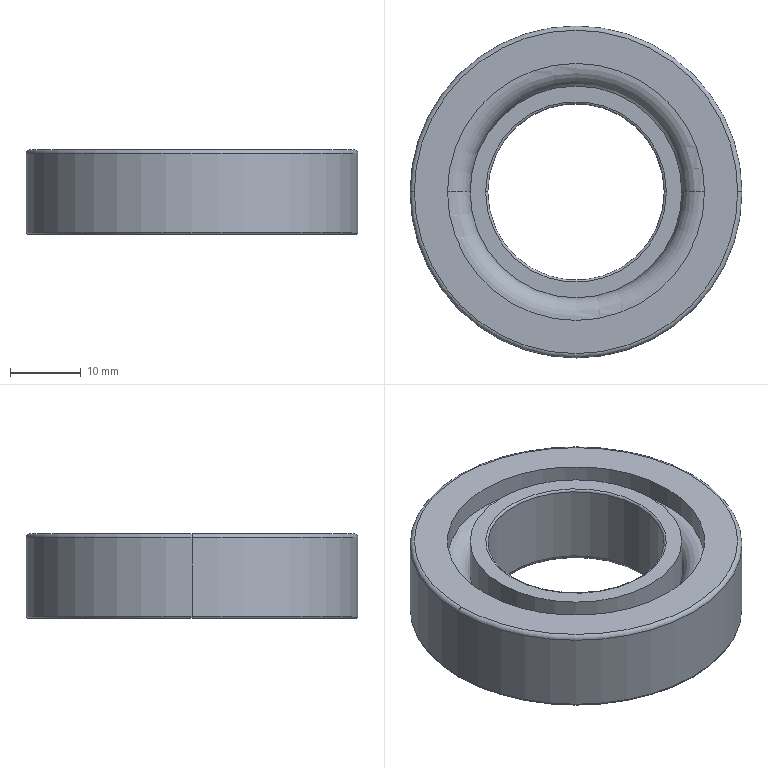Part | SolidWorks | features BaseBody 1 | 1 solid | 28 faces | box 47 x 47 x 12 mm | volume 12629 mm3 | torus 12 | cylinder 12 | plane 4 | commonest cylinder face diameters 25 x2 30 x2 36.4 x2 37.5 x2 42 x2 47 x2
STEP:
#1=CARTESIAN_POINT('',(-23.5,0.,-11.7));
#2=VERTEX_POINT('',#1);
#3=CARTESIAN_POINT('',(23.5,0.,-11.7));
#4=VERTEX_POINT('',#3);
#5=CARTESIAN_POINT('',(0.,0.,-11.7));
#6=DIRECTION('',(0.,0.,-1.));
#7=DIRECTION('',(-1.,0.,0.));
#8=AXIS2_PLACEMENT_3D('',#5,#6,#7);
#9=CIRCLE('',#8,23.5);
#10=EDGE_CURVE('',#2,#4,#9,.T.);
#11=ORIENTED_EDGE('',*,*,#10,.T.);
#12=CARTESIAN_POINT('',(23.2,0.,-12.));
#13=VERTEX_POINT('',#12);
#14=CARTESIAN_POINT('',(23.2,0.,-11.7));
#15=DIRECTION('',(0.,1.,0.));
#16=DIRECTION('',(-1.,0.,0.));
#17=AXIS2_PLACEMENT_3D('',#14,#15,#16);
#18=CIRCLE('',#17,0.3);
#19=EDGE_CURVE('',#4,#13,#18,.T.);
#20=ORIENTED_EDGE('',*,*,#19,.T.);
#21=CARTESIAN_POINT('',(-23.2,0.,-12.));
#22=VERTEX_POINT('',#21);
#23=CARTESIAN_POINT('',(0.,0.,-12.));
#24=DIRECTION('',(0.,0.,-1.));
#25=DIRECTION('',(-1.,0.,0.));
#26=AXIS2_PLACEMENT_3D('',#23,#24,#25);
#27=CIRCLE('',#26,23.2);
#28=EDGE_CURVE('',#22,#13,#27,.T.);
#29=ORIENTED_EDGE('',*,*,#28,.F.);
#30=CARTESIAN_POINT('',(-23.2,0.,-11.7));
#31=DIRECTION('',(0.,-1.,0.));
#32=DIRECTION('',(0.,0.,-1.));
#33=AXIS2_PLACEMENT_3D('',#30,#31,#32);
#34=CIRCLE('',#33,0.3);
#35=EDGE_CURVE('',#2,#22,#34,.T.);
#36=ORIENTED_EDGE('',*,*,#35,.F.);
#37=EDGE_LOOP('',(#11,#20,#29,#36));
#38=FACE_OUTER_BOUND('',#37,.T.);
#39=CARTESIAN_POINT('',(0.,0.,-11.7));
#40=DIRECTION('',(0.,0.,-1.));
#41=DIRECTION('',(-1.,0.,0.));
#42=AXIS2_PLACEMENT_3D('',#39,#40,#41);
#43=TOROIDAL_SURFACE('',#42,23.2,0.3);
#44=ADVANCED_FACE('',(#38),#43,.T.);
#45=CARTESIAN_POINT('',(21.,0.,-6.));
#46=VERTEX_POINT('',#45);
#47=CARTESIAN_POINT('',(-21.,0.,-6.));
#48=VERTEX_POINT('',#47);
#49=CARTESIAN_POINT('',(0.,0.,-6.));
#50=DIRECTION('',(0.,0.,-1.));
#51=DIRECTION('',(-1.,0.,0.));
#52=AXIS2_PLACEMENT_3D('',#49,#50,#51);
#53=CIRCLE('',#52,21.);
#54=EDGE_CURVE('',#46,#48,#53,.T.);
#55=ORIENTED_EDGE('',*,*,#54,.F.);
#56=CARTESIAN_POINT('',(21.,0.,-12.));
#57=VERTEX_POINT('',#56);
#58=CARTESIAN_POINT('',(21.,0.,-12.));
#59=DIRECTION('',(0.,0.,-1.));
#60=VECTOR('',#59,1000.);
#61=LINE('',#58,#60);
#62=EDGE_CURVE('',#46,#57,#61,.T.);
#63=ORIENTED_EDGE('',*,*,#62,.T.);
#64=CARTESIAN_POINT('',(-21.,0.,-12.));
#65=VERTEX_POINT('',#64);
#66=CARTESIAN_POINT('',(0.,0.,-12.));
#67=DIRECTION('',(0.,0.,-1.));
#68=DIRECTION('',(-1.,0.,0.));
#69=AXIS2_PLACEMENT_3D('',#66,#67,#68);
#70=CIRCLE('',#69,21.);
#71=EDGE_CURVE('',#57,#65,#70,.T.);
#72=ORIENTED_EDGE('',*,*,#71,.T.);
#73=CARTESIAN_POINT('',(-21.,0.,-12.));
#74=DIRECTION('',(0.,0.,-1.));
#75=VECTOR('',#74,1000.);
#76=LINE('',#73,#75);
#77=EDGE_CURVE('',#48,#65,#76,.T.);
#78=ORIENTED_EDGE('',*,*,#77,.F.);
#79=EDGE_LOOP('',(#55,#63,#72,#78));
#80=FACE_OUTER_BOUND('',#79,.T.);
#81=CARTESIAN_POINT('',(0.,0.,-12.));
#82=DIRECTION('',(0.,0.,-1.));
#83=DIRECTION('',(-1.,0.,0.));
#84=AXIS2_PLACEMENT_3D('',#81,#82,#83);
#85=CYLINDRICAL_SURFACE('',#84,21.);
#86=ADVANCED_FACE('',(#80),#85,.F.);
#87=CARTESIAN_POINT('',(-23.5,0.,-0.6));
#88=VERTEX_POINT('',#87);
#89=CARTESIAN_POINT('',(23.5,0.,-0.6));
#90=VERTEX_POINT('',#89);
#91=CARTESIAN_POINT('',(0.,0.,-0.6));
#92=DIRECTION('',(0.,0.,-1.));
#93=DIRECTION('',(-1.,0.,0.));
#94=AXIS2_PLACEMENT_3D('',#91,#92,#93);
#95=CIRCLE('',#94,23.5);
#96=EDGE_CURVE('',#88,#90,#95,.T.);
#97=ORIENTED_EDGE('',*,*,#96,.T.);
#98=CARTESIAN_POINT('',(23.5,0.,-12.));
#99=DIRECTION('',(0.,0.,-1.));
#100=VECTOR('',#99,1000.);
#101=LINE('',#98,#100);
#102=EDGE_CURVE('',#90,#4,#101,.T.);
#103=ORIENTED_EDGE('',*,*,#102,.T.);
#104=ORIENTED_EDGE('',*,*,#10,.F.);
#105=CARTESIAN_POINT('',(-23.5,0.,-12.));
#106=DIRECTION('',(0.,0.,-1.));
#107=VECTOR('',#106,1000.);
#108=LINE('',#105,#107);
#109=EDGE_CURVE('',#88,#2,#108,.T.);
#110=ORIENTED_EDGE('',*,*,#109,.F.);
#111=EDGE_LOOP('',(#97,#103,#104,#110));
#112=FACE_OUTER_BOUND('',#111,.T.);
#113=CARTESIAN_POINT('',(0.,0.,-12.));
#114=DIRECTION('',(0.,0.,-1.));
#115=DIRECTION('',(-1.,0.,0.));
#116=AXIS2_PLACEMENT_3D('',#113,#114,#115);
#117=CYLINDRICAL_SURFACE('',#116,23.5);
#118=ADVANCED_FACE('',(#112),#117,.T.);
#119=CARTESIAN_POINT('',(0.,0.,-6.));
#120=DIRECTION('',(0.,0.,-1.));
#121=DIRECTION('',(-1.,0.,0.));
#122=AXIS2_PLACEMENT_3D('',#119,#120,#121);
#123=CIRCLE('',#122,21.);
#124=EDGE_CURVE('',#48,#46,#123,.T.);
#125=ORIENTED_EDGE('',*,*,#124,.T.);
#126=CARTESIAN_POINT('',(18.75,0.,-8.905));
#127=VERTEX_POINT('',#126);
#128=CARTESIAN_POINT('',(18.,0.,-6.));
#129=DIRECTION('',(0.,1.,0.));
#130=DIRECTION('',(-1.,0.,0.));
#131=AXIS2_PLACEMENT_3D('',#128,#129,#130);
#132=CIRCLE('',#131,3.);
#133=EDGE_CURVE('',#46,#127,#132,.T.);
#134=ORIENTED_EDGE('',*,*,#133,.T.);
#135=CARTESIAN_POINT('',(-18.75,0.,-8.905));
#136=VERTEX_POINT('',#135);
#137=CARTESIAN_POINT('',(0.,0.,-8.905));
#138=DIRECTION('',(0.,0.,-1.));
#139=DIRECTION('',(-1.,0.,0.));
#140=AXIS2_PLACEMENT_3D('',#137,#138,#139);
#141=CIRCLE('',#140,18.75);
#142=EDGE_CURVE('',#136,#127,#141,.T.);
#143=ORIENTED_EDGE('',*,*,#142,.F.);
#144=CARTESIAN_POINT('',(-18.,0.,-6.));
#145=DIRECTION('',(0.,-1.,0.));
#146=DIRECTION('',(0.,0.,-1.));
#147=AXIS2_PLACEMENT_3D('',#144,#145,#146);
#148=CIRCLE('',#147,3.);
#149=EDGE_CURVE('',#48,#136,#148,.T.);
#150=ORIENTED_EDGE('',*,*,#149,.F.);
#151=EDGE_LOOP('',(#125,#134,#143,#150));
#152=FACE_OUTER_BOUND('',#151,.T.);
#153=CARTESIAN_POINT('',(0.,0.,-6.));
#154=DIRECTION('',(0.,0.,-1.));
#155=DIRECTION('',(-1.,0.,0.));
#156=AXIS2_PLACEMENT_3D('',#153,#154,#155);
#157=TOROIDAL_SURFACE('',#156,18.,3.);
#158=ADVANCED_FACE('',(#152),#157,.T.);
#159=CARTESIAN_POINT('',(-22.9,0.,0.));
#160=VERTEX_POINT('',#159);
#161=CARTESIAN_POINT('',(22.9,0.,0.));
#162=VERTEX_POINT('',#161);
#163=CARTESIAN_POINT('',(0.,0.,0.));
#164=DIRECTION('',(0.,0.,-1.));
#165=DIRECTION('',(-1.,0.,0.));
#166=AXIS2_PLACEMENT_3D('',#163,#164,#165);
#167=CIRCLE('',#166,22.9);
#168=EDGE_CURVE('',#160,#162,#167,.T.);
#169=ORIENTED_EDGE('',*,*,#168,.T.);
#170=CARTESIAN_POINT('',(22.9,0.,-0.6));
#171=DIRECTION('',(0.,1.,0.));
#172=DIRECTION('',(-1.,0.,0.));
#173=AXIS2_PLACEMENT_3D('',#170,#171,#172);
#174=CIRCLE('',#173,0.6);
#175=EDGE_CURVE('',#162,#90,#174,.T.);
#176=ORIENTED_EDGE('',*,*,#175,.T.);
#177=ORIENTED_EDGE('',*,*,#96,.F.);
#178=CARTESIAN_POINT('',(-22.9,0.,-0.6));
#179=DIRECTION('',(0.,-1.,0.));
#180=DIRECTION('',(0.,0.,-1.));
#181=AXIS2_PLACEMENT_3D('',#178,#179,#180);
#182=CIRCLE('',#181,0.6);
#183=EDGE_CURVE('',#160,#88,#182,.T.);
#184=ORIENTED_EDGE('',*,*,#183,.F.);
#185=EDGE_LOOP('',(#169,#176,#177,#184));
#186=FACE_OUTER_BOUND('',#185,.T.);
#187=CARTESIAN_POINT('',(0.,0.,-0.6));
#188=DIRECTION('',(0.,0.,-1.));
#189=DIRECTION('',(-1.,0.,0.));
#190=AXIS2_PLACEMENT_3D('',#187,#188,#189);
#191=TOROIDAL_SURFACE('',#190,22.9,0.6);
#192=ADVANCED_FACE('',(#186),#191,.T.);
#193=ORIENTED_EDGE('',*,*,#142,.T.);
#194=CARTESIAN_POINT('',(18.75,0.,-12.));
#195=VERTEX_POINT('',#194);
#196=CARTESIAN_POINT('',(18.75,0.,-12.));
#197=DIRECTION('',(0.,0.,-1.));
#198=VECTOR('',#197,1000.);
#199=LINE('',#196,#198);
#200=EDGE_CURVE('',#127,#195,#199,.T.);
#201=ORIENTED_EDGE('',*,*,#200,.T.);
#202=CARTESIAN_POINT('',(-18.75,0.,-12.));
#203=VERTEX_POINT('',#202);
#204=CARTESIAN_POINT('',(0.,0.,-12.));
#205=DIRECTION('',(0.,0.,-1.));
#206=DIRECTION('',(-1.,0.,0.));
#207=AXIS2_PLACEMENT_3D('',#204,#205,#206);
#208=CIRCLE('',#207,18.75);
#209=EDGE_CURVE('',#203,#195,#208,.T.);
#210=ORIENTED_EDGE('',*,*,#209,.F.);
#211=CARTESIAN_POINT('',(-18.75,0.,-12.));
#212=DIRECTION('',(0.,0.,-1.));
#213=VECTOR('',#212,1000.);
#214=LINE('',#211,#213);
#215=EDGE_CURVE('',#136,#203,#214,.T.);
#216=ORIENTED_EDGE('',*,*,#215,.F.);
#217=EDGE_LOOP('',(#193,#201,#210,#216));
#218=FACE_OUTER_BOUND('',#217,.T.);
#219=CARTESIAN_POINT('',(0.,0.,-12.));
#220=DIRECTION('',(0.,0.,-1.));
#221=DIRECTION('',(-1.,0.,0.));
#222=AXIS2_PLACEMENT_3D('',#219,#220,#221);
#223=CYLINDRICAL_SURFACE('',#222,18.75);
#224=ADVANCED_FACE('',(#218),#223,.T.);
#225=CARTESIAN_POINT('',(18.2,0.,0.));
#226=VERTEX_POINT('',#225);
#227=CARTESIAN_POINT('',(-18.2,0.,0.));
#228=VERTEX_POINT('',#227);
#229=CARTESIAN_POINT('',(0.,0.,0.));
#230=DIRECTION('',(0.,0.,-1.));
#231=DIRECTION('',(-1.,0.,0.));
#232=AXIS2_PLACEMENT_3D('',#229,#230,#231);
#233=CIRCLE('',#232,18.2);
#234=EDGE_CURVE('',#226,#228,#233,.T.);
#235=ORIENTED_EDGE('',*,*,#234,.F.);
#236=CARTESIAN_POINT('',(18.2,0.,-3.007));
#237=VERTEX_POINT('',#236);
#238=CARTESIAN_POINT('',(18.2,0.,-12.));
#239=DIRECTION('',(0.,0.,-1.));
#240=VECTOR('',#239,1000.);
#241=LINE('',#238,#240);
#242=EDGE_CURVE('',#226,#237,#241,.T.);
#243=ORIENTED_EDGE('',*,*,#242,.T.);
#244=CARTESIAN_POINT('',(-18.2,0.,-3.007));
#245=VERTEX_POINT('',#244);
#246=CARTESIAN_POINT('',(0.,0.,-3.007));
#247=DIRECTION('',(0.,0.,-1.));
#248=DIRECTION('',(-1.,0.,0.));
#249=AXIS2_PLACEMENT_3D('',#246,#247,#248);
#250=CIRCLE('',#249,18.2);
#251=EDGE_CURVE('',#237,#245,#250,.T.);
#252=ORIENTED_EDGE('',*,*,#251,.T.);
#253=CARTESIAN_POINT('',(-18.2,0.,-12.));
#254=DIRECTION('',(0.,0.,-1.));
#255=VECTOR('',#254,1000.);
#256=LINE('',#253,#255);
#257=EDGE_CURVE('',#228,#245,#256,.T.);
#258=ORIENTED_EDGE('',*,*,#257,.F.);
#259=EDGE_LOOP('',(#235,#243,#252,#258));
#260=FACE_OUTER_BOUND('',#259,.T.);
#261=CARTESIAN_POINT('',(0.,0.,-12.));
#262=DIRECTION('',(0.,0.,-1.));
#263=DIRECTION('',(-1.,0.,0.));
#264=AXIS2_PLACEMENT_3D('',#261,#262,#263);
#265=CYLINDRICAL_SURFACE('',#264,18.2);
#266=ADVANCED_FACE('',(#260),#265,.F.);
#267=CARTESIAN_POINT('',(-13.1,0.,-12.));
#268=VERTEX_POINT('',#267);
#269=CARTESIAN_POINT('',(13.1,0.,-12.));
#270=VERTEX_POINT('',#269);
#271=CARTESIAN_POINT('',(0.,0.,-12.));
#272=DIRECTION('',(0.,0.,-1.));
#273=DIRECTION('',(-1.,0.,0.));
#274=AXIS2_PLACEMENT_3D('',#271,#272,#273);
#275=CIRCLE('',#274,13.1);
#276=EDGE_CURVE('',#268,#270,#275,.T.);
#277=ORIENTED_EDGE('',*,*,#276,.T.);
#278=CARTESIAN_POINT('',(12.5,0.,-11.4));
#279=VERTEX_POINT('',#278);
#280=CARTESIAN_POINT('',(13.1,0.,-11.4));
#281=DIRECTION('',(0.,1.,0.));
#282=DIRECTION('',(-1.,0.,0.));
#283=AXIS2_PLACEMENT_3D('',#280,#281,#282);
#284=CIRCLE('',#283,0.6);
#285=EDGE_CURVE('',#270,#279,#284,.T.);
#286=ORIENTED_EDGE('',*,*,#285,.T.);
#287=CARTESIAN_POINT('',(-12.5,0.,-11.4));
#288=VERTEX_POINT('',#287);
#289=CARTESIAN_POINT('',(0.,0.,-11.4));
#290=DIRECTION('',(0.,0.,-1.));
#291=DIRECTION('',(-1.,0.,0.));
#292=AXIS2_PLACEMENT_3D('',#289,#290,#291);
#293=CIRCLE('',#292,12.5);
#294=EDGE_CURVE('',#288,#279,#293,.T.);
#295=ORIENTED_EDGE('',*,*,#294,.F.);
#296=CARTESIAN_POINT('',(-13.1,0.,-11.4));
#297=DIRECTION('',(0.,-1.,0.));
#298=DIRECTION('',(0.,0.,-1.));
#299=AXIS2_PLACEMENT_3D('',#296,#297,#298);
#300=CIRCLE('',#299,0.6);
#301=EDGE_CURVE('',#268,#288,#300,.T.);
#302=ORIENTED_EDGE('',*,*,#301,.F.);
#303=EDGE_LOOP('',(#277,#286,#295,#302));
#304=FACE_OUTER_BOUND('',#303,.T.);
#305=CARTESIAN_POINT('',(0.,0.,-11.4));
#306=DIRECTION('',(0.,0.,-1.));
#307=DIRECTION('',(-1.,0.,0.));
#308=AXIS2_PLACEMENT_3D('',#305,#306,#307);
#309=TOROIDAL_SURFACE('',#308,13.1,0.6);
#310=ADVANCED_FACE('',(#304),#309,.T.);
#311=CARTESIAN_POINT('',(-15.,0.,-6.));
#312=VERTEX_POINT('',#311);
#313=CARTESIAN_POINT('',(15.,0.,-6.));
#314=VERTEX_POINT('',#313);
#315=CARTESIAN_POINT('',(0.,0.,-6.));
#316=DIRECTION('',(0.,0.,-1.));
#317=DIRECTION('',(-1.,0.,0.));
#318=AXIS2_PLACEMENT_3D('',#315,#316,#317);
#319=CIRCLE('',#318,15.);
#320=EDGE_CURVE('',#312,#314,#319,.T.);
#321=ORIENTED_EDGE('',*,*,#320,.T.);
#322=CARTESIAN_POINT('',(18.,0.,-6.));
#323=DIRECTION('',(0.,1.,0.));
#324=DIRECTION('',(-1.,0.,0.));
#325=AXIS2_PLACEMENT_3D('',#322,#323,#324);
#326=CIRCLE('',#325,3.);
#327=EDGE_CURVE('',#314,#237,#326,.T.);
#328=ORIENTED_EDGE('',*,*,#327,.T.);
#329=CARTESIAN_POINT('',(0.,0.,-3.007));
#330=DIRECTION('',(0.,0.,-1.));
#331=DIRECTION('',(-1.,0.,0.));
#332=AXIS2_PLACEMENT_3D('',#329,#330,#331);
#333=CIRCLE('',#332,18.2);
#334=EDGE_CURVE('',#245,#237,#333,.T.);
#335=ORIENTED_EDGE('',*,*,#334,.F.);
#336=CARTESIAN_POINT('',(-18.,0.,-6.));
#337=DIRECTION('',(0.,-1.,0.));
#338=DIRECTION('',(0.,0.,-1.));
#339=AXIS2_PLACEMENT_3D('',#336,#337,#338);
#340=CIRCLE('',#339,3.);
#341=EDGE_CURVE('',#312,#245,#340,.T.);
#342=ORIENTED_EDGE('',*,*,#341,.F.);
#343=EDGE_LOOP('',(#321,#328,#335,#342));
#344=FACE_OUTER_BOUND('',#343,.T.);
#345=CARTESIAN_POINT('',(0.,0.,-6.));
#346=DIRECTION('',(0.,0.,-1.));
#347=DIRECTION('',(-1.,0.,0.));
#348=AXIS2_PLACEMENT_3D('',#345,#346,#347);
#349=TOROIDAL_SURFACE('',#348,18.,3.);
#350=ADVANCED_FACE('',(#344),#349,.T.);
#351=CARTESIAN_POINT('',(12.5,0.,-0.3));
#352=VERTEX_POINT('',#351);
#353=CARTESIAN_POINT('',(-12.5,0.,-0.3));
#354=VERTEX_POINT('',#353);
#355=CARTESIAN_POINT('',(0.,0.,-0.3));
#356=DIRECTION('',(0.,0.,-1.));
#357=DIRECTION('',(-1.,0.,0.));
#358=AXIS2_PLACEMENT_3D('',#355,#356,#357);
#359=CIRCLE('',#358,12.5);
#360=EDGE_CURVE('',#352,#354,#359,.T.);
#361=ORIENTED_EDGE('',*,*,#360,.F.);
#362=CARTESIAN_POINT('',(12.5,0.,-12.));
#363=DIRECTION('',(0.,0.,-1.));
#364=VECTOR('',#363,1000.);
#365=LINE('',#362,#364);
#366=EDGE_CURVE('',#352,#279,#365,.T.);
#367=ORIENTED_EDGE('',*,*,#366,.T.);
#368=CARTESIAN_POINT('',(0.,0.,-11.4));
#369=DIRECTION('',(0.,0.,-1.));
#370=DIRECTION('',(-1.,0.,0.));
#371=AXIS2_PLACEMENT_3D('',#368,#369,#370);
#372=CIRCLE('',#371,12.5);
#373=EDGE_CURVE('',#279,#288,#372,.T.);
#374=ORIENTED_EDGE('',*,*,#373,.T.);
#375=CARTESIAN_POINT('',(-12.5,0.,-12.));
#376=DIRECTION('',(0.,0.,-1.));
#377=VECTOR('',#376,1000.);
#378=LINE('',#375,#377);
#379=EDGE_CURVE('',#354,#288,#378,.T.);
#380=ORIENTED_EDGE('',*,*,#379,.F.);
#381=EDGE_LOOP('',(#361,#367,#374,#380));
#382=FACE_OUTER_BOUND('',#381,.T.);
#383=CARTESIAN_POINT('',(0.,0.,-12.));
#384=DIRECTION('',(0.,0.,-1.));
#385=DIRECTION('',(-1.,0.,0.));
#386=AXIS2_PLACEMENT_3D('',#383,#384,#385);
#387=CYLINDRICAL_SURFACE('',#386,12.5);
#388=ADVANCED_FACE('',(#382),#387,.F.);
#389=CARTESIAN_POINT('',(-15.,0.,0.));
#390=VERTEX_POINT('',#389);
#391=CARTESIAN_POINT('',(15.,0.,0.));
#392=VERTEX_POINT('',#391);
#393=CARTESIAN_POINT('',(0.,0.,0.));
#394=DIRECTION('',(0.,0.,-1.));
#395=DIRECTION('',(-1.,0.,0.));
#396=AXIS2_PLACEMENT_3D('',#393,#394,#395);
#397=CIRCLE('',#396,15.);
#398=EDGE_CURVE('',#390,#392,#397,.T.);
#399=ORIENTED_EDGE('',*,*,#398,.T.);
#400=CARTESIAN_POINT('',(15.,0.,-12.));
#401=DIRECTION('',(0.,0.,-1.));
#402=VECTOR('',#401,1000.);
#403=LINE('',#400,#402);
#404=EDGE_CURVE('',#392,#314,#403,.T.);
#405=ORIENTED_EDGE('',*,*,#404,.T.);
#406=ORIENTED_EDGE('',*,*,#320,.F.);
#407=CARTESIAN_POINT('',(-15.,0.,-12.));
#408=DIRECTION('',(0.,0.,-1.));
#409=VECTOR('',#408,1000.);
#410=LINE('',#407,#409);
#411=EDGE_CURVE('',#390,#312,#410,.T.);
#412=ORIENTED_EDGE('',*,*,#411,.F.);
#413=EDGE_LOOP('',(#399,#405,#406,#412));
#414=FACE_OUTER_BOUND('',#413,.T.);
#415=CARTESIAN_POINT('',(0.,0.,-12.));
#416=DIRECTION('',(0.,0.,-1.));
#417=DIRECTION('',(-1.,0.,0.));
#418=AXIS2_PLACEMENT_3D('',#415,#416,#417);
#419=CYLINDRICAL_SURFACE('',#418,15.);
#420=ADVANCED_FACE('',(#414),#419,.T.);
#421=CARTESIAN_POINT('',(0.,0.,-0.3));
#422=DIRECTION('',(0.,0.,-1.));
#423=DIRECTION('',(-1.,0.,0.));
#424=AXIS2_PLACEMENT_3D('',#421,#422,#423);
#425=CIRCLE('',#424,12.5);
#426=EDGE_CURVE('',#354,#352,#425,.T.);
#427=ORIENTED_EDGE('',*,*,#426,.T.);
#428=CARTESIAN_POINT('',(12.8,0.,0.));
#429=VERTEX_POINT('',#428);
#430=CARTESIAN_POINT('',(12.8,0.,-0.3));
#431=DIRECTION('',(0.,1.,0.));
#432=DIRECTION('',(-1.,0.,0.));
#433=AXIS2_PLACEMENT_3D('',#430,#431,#432);
#434=CIRCLE('',#433,0.3);
#435=EDGE_CURVE('',#352,#429,#434,.T.);
#436=ORIENTED_EDGE('',*,*,#435,.T.);
#437=CARTESIAN_POINT('',(-12.8,0.,0.));
#438=VERTEX_POINT('',#437);
#439=CARTESIAN_POINT('',(0.,0.,0.));
#440=DIRECTION('',(0.,0.,-1.));
#441=DIRECTION('',(-1.,0.,0.));
#442=AXIS2_PLACEMENT_3D('',#439,#440,#441);
#443=CIRCLE('',#442,12.8);
#444=EDGE_CURVE('',#438,#429,#443,.T.);
#445=ORIENTED_EDGE('',*,*,#444,.F.);
#446=CARTESIAN_POINT('',(-12.8,0.,-0.3));
#447=DIRECTION('',(0.,-1.,0.));
#448=DIRECTION('',(0.,0.,-1.));
#449=AXIS2_PLACEMENT_3D('',#446,#447,#448);
#450=CIRCLE('',#449,0.3);
#451=EDGE_CURVE('',#354,#438,#450,.T.);
#452=ORIENTED_EDGE('',*,*,#451,.F.);
#453=EDGE_LOOP('',(#427,#436,#445,#452));
#454=FACE_OUTER_BOUND('',#453,.T.);
#455=CARTESIAN_POINT('',(0.,0.,-0.3));
#456=DIRECTION('',(0.,0.,-1.));
#457=DIRECTION('',(-1.,0.,0.));
#458=AXIS2_PLACEMENT_3D('',#455,#456,#457);
#459=TOROIDAL_SURFACE('',#458,12.8,0.3);
#460=ADVANCED_FACE('',(#454),#459,.T.);
#461=ORIENTED_EDGE('',*,*,#444,.T.);
#462=CARTESIAN_POINT('',(0.,0.,0.));
#463=DIRECTION('',(0.,0.,-1.));
#464=DIRECTION('',(-1.,0.,0.));
#465=AXIS2_PLACEMENT_3D('',#462,#463,#464);
#466=CIRCLE('',#465,12.8);
#467=EDGE_CURVE('',#429,#438,#466,.T.);
#468=ORIENTED_EDGE('',*,*,#467,.T.);
#469=EDGE_LOOP('',(#461,#468));
#470=FACE_BOUND('',#469,.T.);
#471=ORIENTED_EDGE('',*,*,#398,.F.);
#472=CARTESIAN_POINT('',(0.,0.,0.));
#473=DIRECTION('',(0.,0.,-1.));
#474=DIRECTION('',(-1.,0.,0.));
#475=AXIS2_PLACEMENT_3D('',#472,#473,#474);
#476=CIRCLE('',#475,15.);
#477=EDGE_CURVE('',#392,#390,#476,.T.);
#478=ORIENTED_EDGE('',*,*,#477,.F.);
#479=EDGE_LOOP('',(#471,#478));
#480=FACE_OUTER_BOUND('',#479,.T.);
#481=CARTESIAN_POINT('',(0.,15.,0.));
#482=DIRECTION('',(0.,0.,1.));
#483=DIRECTION('',(1.,0.,0.));
#484=AXIS2_PLACEMENT_3D('',#481,#482,#483);
#485=PLANE('',#484);
#486=ADVANCED_FACE('',(#470,#480),#485,.T.);
#487=ORIENTED_EDGE('',*,*,#435,.F.);
#488=ORIENTED_EDGE('',*,*,#360,.T.);
#489=ORIENTED_EDGE('',*,*,#451,.T.);
#490=ORIENTED_EDGE('',*,*,#467,.F.);
#491=EDGE_LOOP('',(#487,#488,#489,#490));
#492=FACE_OUTER_BOUND('',#491,.T.);
#493=CARTESIAN_POINT('',(0.,0.,-0.3));
#494=DIRECTION('',(0.,0.,-1.));
#495=DIRECTION('',(-1.,0.,0.));
#496=AXIS2_PLACEMENT_3D('',#493,#494,#495);
#497=TOROIDAL_SURFACE('',#496,12.8,0.3);
#498=ADVANCED_FACE('',(#492),#497,.T.);
#499=ORIENTED_EDGE('',*,*,#404,.F.);
#500=ORIENTED_EDGE('',*,*,#477,.T.);
#501=ORIENTED_EDGE('',*,*,#411,.T.);
#502=CARTESIAN_POINT('',(0.,0.,-6.));
#503=DIRECTION('',(0.,0.,-1.));
#504=DIRECTION('',(-1.,0.,0.));
#505=AXIS2_PLACEMENT_3D('',#502,#503,#504);
#506=CIRCLE('',#505,15.);
#507=EDGE_CURVE('',#314,#312,#506,.T.);
#508=ORIENTED_EDGE('',*,*,#507,.F.);
#509=EDGE_LOOP('',(#499,#500,#501,#508));
#510=FACE_OUTER_BOUND('',#509,.T.);
#511=CARTESIAN_POINT('',(0.,0.,-12.));
#512=DIRECTION('',(0.,0.,-1.));
#513=DIRECTION('',(-1.,0.,0.));
#514=AXIS2_PLACEMENT_3D('',#511,#512,#513);
#515=CYLINDRICAL_SURFACE('',#514,15.);
#516=ADVANCED_FACE('',(#510),#515,.T.);
#517=ORIENTED_EDGE('',*,*,#366,.F.);
#518=ORIENTED_EDGE('',*,*,#426,.F.);
#519=ORIENTED_EDGE('',*,*,#379,.T.);
#520=ORIENTED_EDGE('',*,*,#294,.T.);
#521=EDGE_LOOP('',(#517,#518,#519,#520));
#522=FACE_OUTER_BOUND('',#521,.T.);
#523=CARTESIAN_POINT('',(0.,0.,-12.));
#524=DIRECTION('',(0.,0.,-1.));
#525=DIRECTION('',(-1.,0.,0.));
#526=AXIS2_PLACEMENT_3D('',#523,#524,#525);
#527=CYLINDRICAL_SURFACE('',#526,12.5);
#528=ADVANCED_FACE('',(#522),#527,.F.);
#529=ORIENTED_EDGE('',*,*,#327,.F.);
#530=ORIENTED_EDGE('',*,*,#507,.T.);
#531=ORIENTED_EDGE('',*,*,#341,.T.);
#532=ORIENTED_EDGE('',*,*,#251,.F.);
#533=EDGE_LOOP('',(#529,#530,#531,#532));
#534=FACE_OUTER_BOUND('',#533,.T.);
#535=CARTESIAN_POINT('',(0.,0.,-6.));
#536=DIRECTION('',(0.,0.,-1.));
#537=DIRECTION('',(-1.,0.,0.));
#538=AXIS2_PLACEMENT_3D('',#535,#536,#537);
#539=TOROIDAL_SURFACE('',#538,18.,3.);
#540=ADVANCED_FACE('',(#534),#539,.T.);
#541=ORIENTED_EDGE('',*,*,#285,.F.);
#542=CARTESIAN_POINT('',(0.,0.,-12.));
#543=DIRECTION('',(0.,0.,-1.));
#544=DIRECTION('',(-1.,0.,0.));
#545=AXIS2_PLACEMENT_3D('',#542,#543,#544);
#546=CIRCLE('',#545,13.1);
#547=EDGE_CURVE('',#270,#268,#546,.T.);
#548=ORIENTED_EDGE('',*,*,#547,.T.);
#549=ORIENTED_EDGE('',*,*,#301,.T.);
#550=ORIENTED_EDGE('',*,*,#373,.F.);
#551=EDGE_LOOP('',(#541,#548,#549,#550));
#552=FACE_OUTER_BOUND('',#551,.T.);
#553=CARTESIAN_POINT('',(0.,0.,-11.4));
#554=DIRECTION('',(0.,0.,-1.));
#555=DIRECTION('',(-1.,0.,0.));
#556=AXIS2_PLACEMENT_3D('',#553,#554,#555);
#557=TOROIDAL_SURFACE('',#556,13.1,0.6);
#558=ADVANCED_FACE('',(#552),#557,.T.);
#559=ORIENTED_EDGE('',*,*,#242,.F.);
#560=CARTESIAN_POINT('',(0.,0.,0.));
#561=DIRECTION('',(0.,0.,-1.));
#562=DIRECTION('',(-1.,0.,0.));
#563=AXIS2_PLACEMENT_3D('',#560,#561,#562);
#564=CIRCLE('',#563,18.2);
#565=EDGE_CURVE('',#228,#226,#564,.T.);
#566=ORIENTED_EDGE('',*,*,#565,.F.);
#567=ORIENTED_EDGE('',*,*,#257,.T.);
#568=ORIENTED_EDGE('',*,*,#334,.T.);
#569=EDGE_LOOP('',(#559,#566,#567,#568));
#570=FACE_OUTER_BOUND('',#569,.T.);
#571=CARTESIAN_POINT('',(0.,0.,-12.));
#572=DIRECTION('',(0.,0.,-1.));
#573=DIRECTION('',(-1.,0.,0.));
#574=AXIS2_PLACEMENT_3D('',#571,#572,#573);
#575=CYLINDRICAL_SURFACE('',#574,18.2);
#576=ADVANCED_FACE('',(#570),#575,.F.);
#577=ORIENTED_EDGE('',*,*,#209,.T.);
#578=CARTESIAN_POINT('',(0.,0.,-12.));
#579=DIRECTION('',(0.,0.,-1.));
#580=DIRECTION('',(-1.,0.,0.));
#581=AXIS2_PLACEMENT_3D('',#578,#579,#580);
#582=CIRCLE('',#581,18.75);
#583=EDGE_CURVE('',#195,#203,#582,.T.);
#584=ORIENTED_EDGE('',*,*,#583,.T.);
#585=EDGE_LOOP('',(#577,#584));
#586=FACE_OUTER_BOUND('',#585,.T.);
#587=ORIENTED_EDGE('',*,*,#276,.F.);
#588=ORIENTED_EDGE('',*,*,#547,.F.);
#589=EDGE_LOOP('',(#587,#588));
#590=FACE_BOUND('',#589,.T.);
#591=CARTESIAN_POINT('',(0.,13.1,-12.));
#592=DIRECTION('',(0.,0.,-1.));
#593=DIRECTION('',(-1.,0.,0.));
#594=AXIS2_PLACEMENT_3D('',#591,#592,#593);
#595=PLANE('',#594);
#596=ADVANCED_FACE('',(#586,#590),#595,.T.);
#597=ORIENTED_EDGE('',*,*,#565,.T.);
#598=ORIENTED_EDGE('',*,*,#234,.T.);
#599=EDGE_LOOP('',(#597,#598));
#600=FACE_BOUND('',#599,.T.);
#601=ORIENTED_EDGE('',*,*,#168,.F.);
#602=CARTESIAN_POINT('',(0.,0.,0.));
#603=DIRECTION('',(0.,0.,-1.));
#604=DIRECTION('',(-1.,0.,0.));
#605=AXIS2_PLACEMENT_3D('',#602,#603,#604);
#606=CIRCLE('',#605,22.9);
#607=EDGE_CURVE('',#162,#160,#606,.T.);
#608=ORIENTED_EDGE('',*,*,#607,.F.);
#609=EDGE_LOOP('',(#601,#608));
#610=FACE_OUTER_BOUND('',#609,.T.);
#611=CARTESIAN_POINT('',(0.,22.9,0.));
#612=DIRECTION('',(0.,0.,1.));
#613=DIRECTION('',(1.,0.,0.));
#614=AXIS2_PLACEMENT_3D('',#611,#612,#613);
#615=PLANE('',#614);
#616=ADVANCED_FACE('',(#600,#610),#615,.T.);
#617=ORIENTED_EDGE('',*,*,#200,.F.);
#618=CARTESIAN_POINT('',(0.,0.,-8.905));
#619=DIRECTION('',(0.,0.,-1.));
#620=DIRECTION('',(-1.,0.,0.));
#621=AXIS2_PLACEMENT_3D('',#618,#619,#620);
#622=CIRCLE('',#621,18.75);
#623=EDGE_CURVE('',#127,#136,#622,.T.);
#624=ORIENTED_EDGE('',*,*,#623,.T.);
#625=ORIENTED_EDGE('',*,*,#215,.T.);
#626=ORIENTED_EDGE('',*,*,#583,.F.);
#627=EDGE_LOOP('',(#617,#624,#625,#626));
#628=FACE_OUTER_BOUND('',#627,.T.);
#629=CARTESIAN_POINT('',(0.,0.,-12.));
#630=DIRECTION('',(0.,0.,-1.));
#631=DIRECTION('',(-1.,0.,0.));
#632=AXIS2_PLACEMENT_3D('',#629,#630,#631);
#633=CYLINDRICAL_SURFACE('',#632,18.75);
#634=ADVANCED_FACE('',(#628),#633,.T.);
#635=ORIENTED_EDGE('',*,*,#175,.F.);
#636=ORIENTED_EDGE('',*,*,#607,.T.);
#637=ORIENTED_EDGE('',*,*,#183,.T.);
#638=CARTESIAN_POINT('',(0.,0.,-0.6));
#639=DIRECTION('',(0.,0.,-1.));
#640=DIRECTION('',(-1.,0.,0.));
#641=AXIS2_PLACEMENT_3D('',#638,#639,#640);
#642=CIRCLE('',#641,23.5);
#643=EDGE_CURVE('',#90,#88,#642,.T.);
#644=ORIENTED_EDGE('',*,*,#643,.F.);
#645=EDGE_LOOP('',(#635,#636,#637,#644));
#646=FACE_OUTER_BOUND('',#645,.T.);
#647=CARTESIAN_POINT('',(0.,0.,-0.6));
#648=DIRECTION('',(0.,0.,-1.));
#649=DIRECTION('',(-1.,0.,0.));
#650=AXIS2_PLACEMENT_3D('',#647,#648,#649);
#651=TOROIDAL_SURFACE('',#650,22.9,0.6);
#652=ADVANCED_FACE('',(#646),#651,.T.);
#653=ORIENTED_EDGE('',*,*,#133,.F.);
#654=ORIENTED_EDGE('',*,*,#54,.T.);
#655=ORIENTED_EDGE('',*,*,#149,.T.);
#656=ORIENTED_EDGE('',*,*,#623,.F.);
#657=EDGE_LOOP('',(#653,#654,#655,#656));
#658=FACE_OUTER_BOUND('',#657,.T.);
#659=CARTESIAN_POINT('',(0.,0.,-6.));
#660=DIRECTION('',(0.,0.,-1.));
#661=DIRECTION('',(-1.,0.,0.));
#662=AXIS2_PLACEMENT_3D('',#659,#660,#661);
#663=TOROIDAL_SURFACE('',#662,18.,3.);
#664=ADVANCED_FACE('',(#658),#663,.T.);
#665=ORIENTED_EDGE('',*,*,#102,.F.);
#666=ORIENTED_EDGE('',*,*,#643,.T.);
#667=ORIENTED_EDGE('',*,*,#109,.T.);
#668=CARTESIAN_POINT('',(0.,0.,-11.7));
#669=DIRECTION('',(0.,0.,-1.));
#670=DIRECTION('',(-1.,0.,0.));
#671=AXIS2_PLACEMENT_3D('',#668,#669,#670);
#672=CIRCLE('',#671,23.5);
#673=EDGE_CURVE('',#4,#2,#672,.T.);
#674=ORIENTED_EDGE('',*,*,#673,.F.);
#675=EDGE_LOOP('',(#665,#666,#667,#674));
#676=FACE_OUTER_BOUND('',#675,.T.);
#677=CARTESIAN_POINT('',(0.,0.,-12.));
#678=DIRECTION('',(0.,0.,-1.));
#679=DIRECTION('',(-1.,0.,0.));
#680=AXIS2_PLACEMENT_3D('',#677,#678,#679);
#681=CYLINDRICAL_SURFACE('',#680,23.5);
#682=ADVANCED_FACE('',(#676),#681,.T.);
#683=ORIENTED_EDGE('',*,*,#62,.F.);
#684=ORIENTED_EDGE('',*,*,#124,.F.);
#685=ORIENTED_EDGE('',*,*,#77,.T.);
#686=CARTESIAN_POINT('',(0.,0.,-12.));
#687=DIRECTION('',(0.,0.,-1.));
#688=DIRECTION('',(-1.,0.,0.));
#689=AXIS2_PLACEMENT_3D('',#686,#687,#688);
#690=CIRCLE('',#689,21.);
#691=EDGE_CURVE('',#65,#57,#690,.T.);
#692=ORIENTED_EDGE('',*,*,#691,.T.);
#693=EDGE_LOOP('',(#683,#684,#685,#692));
#694=FACE_OUTER_BOUND('',#693,.T.);
#695=CARTESIAN_POINT('',(0.,0.,-12.));
#696=DIRECTION('',(0.,0.,-1.));
#697=DIRECTION('',(-1.,0.,0.));
#698=AXIS2_PLACEMENT_3D('',#695,#696,#697);
#699=CYLINDRICAL_SURFACE('',#698,21.);
#700=ADVANCED_FACE('',(#694),#699,.F.);
#701=ORIENTED_EDGE('',*,*,#19,.F.);
#702=ORIENTED_EDGE('',*,*,#673,.T.);
#703=ORIENTED_EDGE('',*,*,#35,.T.);
#704=CARTESIAN_POINT('',(0.,0.,-12.));
#705=DIRECTION('',(0.,0.,-1.));
#706=DIRECTION('',(-1.,0.,0.));
#707=AXIS2_PLACEMENT_3D('',#704,#705,#706);
#708=CIRCLE('',#707,23.2);
#709=EDGE_CURVE('',#13,#22,#708,.T.);
#710=ORIENTED_EDGE('',*,*,#709,.F.);
#711=EDGE_LOOP('',(#701,#702,#703,#710));
#712=FACE_OUTER_BOUND('',#711,.T.);
#713=CARTESIAN_POINT('',(0.,0.,-11.7));
#714=DIRECTION('',(0.,0.,-1.));
#715=DIRECTION('',(-1.,0.,0.));
#716=AXIS2_PLACEMENT_3D('',#713,#714,#715);
#717=TOROIDAL_SURFACE('',#716,23.2,0.3);
#718=ADVANCED_FACE('',(#712),#717,.T.);
#719=ORIENTED_EDGE('',*,*,#28,.T.);
#720=ORIENTED_EDGE('',*,*,#709,.T.);
#721=EDGE_LOOP('',(#719,#720));
#722=FACE_OUTER_BOUND('',#721,.T.);
#723=ORIENTED_EDGE('',*,*,#691,.F.);
#724=ORIENTED_EDGE('',*,*,#71,.F.);
#725=EDGE_LOOP('',(#723,#724));
#726=FACE_BOUND('',#725,.T.);
#727=CARTESIAN_POINT('',(0.,21.,-12.));
#728=DIRECTION('',(0.,0.,-1.));
#729=DIRECTION('',(-1.,0.,0.));
#730=AXIS2_PLACEMENT_3D('',#727,#728,#729);
#731=PLANE('',#730);
#732=ADVANCED_FACE('',(#722,#726),#731,.T.);
#733=CLOSED_SHELL('',(#44,#86,#118,#158,#192,#224,#266,#310,#350,#388,#420,#460,#486,#498,#516,#528,#540,#558,#576,#596,#616,#634,#652,#664,#682,#700,#718,#732));
#734=MANIFOLD_SOLID_BREP('',#733);
#735=CARTESIAN_POINT('',(0.,0.,0.));
#736=DIRECTION('',(0.,0.,1.));
#737=DIRECTION('',(1.,0.,0.));
#738=AXIS2_PLACEMENT_3D('',#735,#736,#737);
#739=(LENGTH_UNIT()NAMED_UNIT(*)SI_UNIT(.MILLI.,.METRE.));
#740=UNCERTAINTY_MEASURE_WITH_UNIT(LENGTH_MEASURE(0.00001),#739,'','');
#741=(NAMED_UNIT(*)PLANE_ANGLE_UNIT()SI_UNIT($,.RADIAN.));
#742=(NAMED_UNIT(*)SI_UNIT($,.STERADIAN.)SOLID_ANGLE_UNIT());
#743=(GEOMETRIC_REPRESENTATION_CONTEXT(3)GLOBAL_UNCERTAINTY_ASSIGNED_CONTEXT((#740))GLOBAL_UNIT_ASSIGNED_CONTEXT((#739,#741,#742))REPRESENTATION_CONTEXT('',''));
#744=ADVANCED_BREP_SHAPE_REPRESENTATION('',(#734,#738),#743);